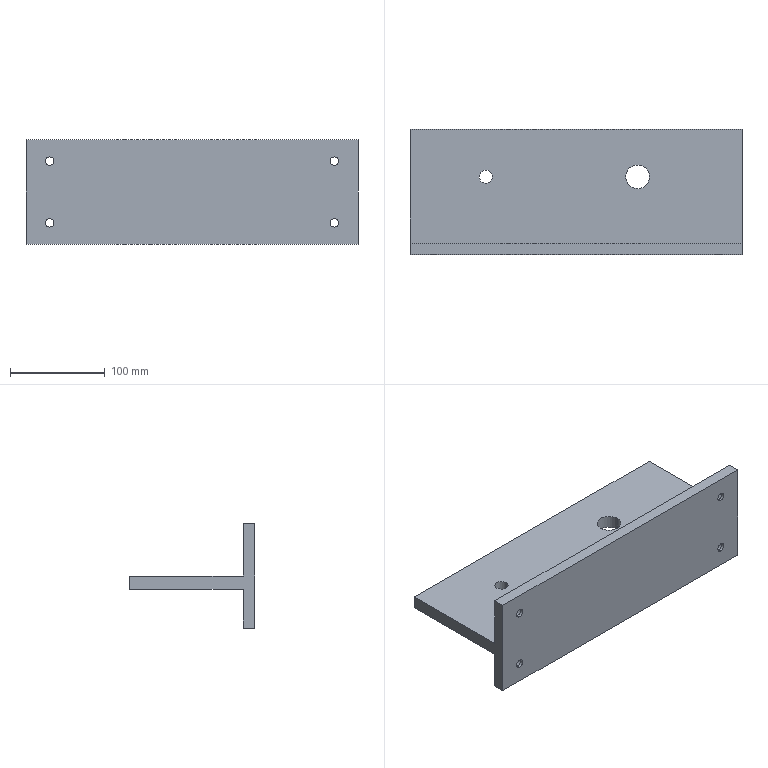Part | SolidWorks | features Cut 2, Extrusion 1, HoleWzd 1, ICE 1 | 1 solid | 42 faces | box 350 x 132 x 110 mm | volume 1033847 mm3 | cylinder 20 | plane 14 | cone 8 | commonest cylinder face diameters 9 x8 15 x8 14 x2 25 x2
STEP:
#1=CARTESIAN_POINT('',(77.5,82.,0.));
#2=VERTEX_POINT('',#1);
#3=CARTESIAN_POINT('',(52.5,82.,0.));
#4=VERTEX_POINT('',#3);
#5=CARTESIAN_POINT('',(65.,82.,0.));
#6=DIRECTION('',(0.,0.,-1.));
#7=DIRECTION('',(-1.,0.,0.));
#8=AXIS2_PLACEMENT_3D('',#5,#6,#7);
#9=CIRCLE('',#8,12.5);
#10=EDGE_CURVE('',#2,#4,#9,.T.);
#11=ORIENTED_EDGE('',*,*,#10,.F.);
#12=CARTESIAN_POINT('',(77.5,82.,-14.));
#13=VERTEX_POINT('',#12);
#14=CARTESIAN_POINT('',(77.5,82.,55.));
#15=DIRECTION('',(0.,0.,-1.));
#16=VECTOR('',#15,1000.);
#17=LINE('',#14,#16);
#18=EDGE_CURVE('',#2,#13,#17,.T.);
#19=ORIENTED_EDGE('',*,*,#18,.T.);
#20=CARTESIAN_POINT('',(52.5,82.,-14.));
#21=VERTEX_POINT('',#20);
#22=CARTESIAN_POINT('',(65.,82.,-14.));
#23=DIRECTION('',(0.,0.,1.));
#24=DIRECTION('',(1.,0.,0.));
#25=AXIS2_PLACEMENT_3D('',#22,#23,#24);
#26=CIRCLE('',#25,12.5);
#27=EDGE_CURVE('',#21,#13,#26,.T.);
#28=ORIENTED_EDGE('',*,*,#27,.F.);
#29=CARTESIAN_POINT('',(52.5,82.,55.));
#30=DIRECTION('',(0.,0.,-1.));
#31=VECTOR('',#30,1000.);
#32=LINE('',#29,#31);
#33=EDGE_CURVE('',#4,#21,#32,.T.);
#34=ORIENTED_EDGE('',*,*,#33,.F.);
#35=EDGE_LOOP('',(#11,#19,#28,#34));
#36=FACE_OUTER_BOUND('',#35,.T.);
#37=CARTESIAN_POINT('',(65.,82.,55.));
#38=DIRECTION('',(0.,0.,-1.));
#39=DIRECTION('',(-1.,0.,0.));
#40=AXIS2_PLACEMENT_3D('',#37,#38,#39);
#41=CYLINDRICAL_SURFACE('',#40,12.5);
#42=ADVANCED_FACE('',(#36),#41,.F.);
#43=CARTESIAN_POINT('',(-88.,82.,0.));
#44=VERTEX_POINT('',#43);
#45=CARTESIAN_POINT('',(-102.,82.,0.));
#46=VERTEX_POINT('',#45);
#47=CARTESIAN_POINT('',(-95.,82.,0.));
#48=DIRECTION('',(0.,0.,-1.));
#49=DIRECTION('',(-1.,0.,0.));
#50=AXIS2_PLACEMENT_3D('',#47,#48,#49);
#51=CIRCLE('',#50,7.);
#52=EDGE_CURVE('',#44,#46,#51,.T.);
#53=ORIENTED_EDGE('',*,*,#52,.F.);
#54=CARTESIAN_POINT('',(-88.,82.,-14.));
#55=VERTEX_POINT('',#54);
#56=CARTESIAN_POINT('',(-88.,82.,55.));
#57=DIRECTION('',(0.,0.,-1.));
#58=VECTOR('',#57,1000.);
#59=LINE('',#56,#58);
#60=EDGE_CURVE('',#44,#55,#59,.T.);
#61=ORIENTED_EDGE('',*,*,#60,.T.);
#62=CARTESIAN_POINT('',(-102.,82.,-14.));
#63=VERTEX_POINT('',#62);
#64=CARTESIAN_POINT('',(-95.,82.,-14.));
#65=DIRECTION('',(0.,0.,1.));
#66=DIRECTION('',(1.,0.,0.));
#67=AXIS2_PLACEMENT_3D('',#64,#65,#66);
#68=CIRCLE('',#67,7.);
#69=EDGE_CURVE('',#63,#55,#68,.T.);
#70=ORIENTED_EDGE('',*,*,#69,.F.);
#71=CARTESIAN_POINT('',(-102.,82.,55.));
#72=DIRECTION('',(0.,0.,-1.));
#73=VECTOR('',#72,1000.);
#74=LINE('',#71,#73);
#75=EDGE_CURVE('',#46,#63,#74,.T.);
#76=ORIENTED_EDGE('',*,*,#75,.F.);
#77=EDGE_LOOP('',(#53,#61,#70,#76));
#78=FACE_OUTER_BOUND('',#77,.T.);
#79=CARTESIAN_POINT('',(-95.,82.,55.));
#80=DIRECTION('',(0.,0.,-1.));
#81=DIRECTION('',(-1.,0.,0.));
#82=AXIS2_PLACEMENT_3D('',#79,#80,#81);
#83=CYLINDRICAL_SURFACE('',#82,7.);
#84=ADVANCED_FACE('',(#78),#83,.F.);
#85=CARTESIAN_POINT('',(-150.,11.975,-40.));
#86=VERTEX_POINT('',#85);
#87=CARTESIAN_POINT('',(-150.,11.975,-25.));
#88=VERTEX_POINT('',#87);
#89=CARTESIAN_POINT('',(-150.,11.975,-32.5));
#90=DIRECTION('',(0.,1.,0.));
#91=DIRECTION('',(0.,0.,1.));
#92=AXIS2_PLACEMENT_3D('',#89,#90,#91);
#93=CIRCLE('',#92,7.5);
#94=EDGE_CURVE('',#86,#88,#93,.T.);
#95=ORIENTED_EDGE('',*,*,#94,.F.);
#96=CARTESIAN_POINT('',(-150.,12.,-40.025));
#97=VERTEX_POINT('',#96);
#98=CARTESIAN_POINT('',(-150.,12.,-40.025));
#99=DIRECTION('',(0.,0.7071,-0.7071));
#100=VECTOR('',#99,1000.);
#101=LINE('',#98,#100);
#102=EDGE_CURVE('',#86,#97,#101,.T.);
#103=ORIENTED_EDGE('',*,*,#102,.T.);
#104=CARTESIAN_POINT('',(-150.,12.,-24.975));
#105=VERTEX_POINT('',#104);
#106=CARTESIAN_POINT('',(-150.,12.,-32.5));
#107=DIRECTION('',(0.,1.,0.));
#108=DIRECTION('',(0.,0.,1.));
#109=AXIS2_PLACEMENT_3D('',#106,#107,#108);
#110=CIRCLE('',#109,7.525);
#111=EDGE_CURVE('',#97,#105,#110,.T.);
#112=ORIENTED_EDGE('',*,*,#111,.T.);
#113=CARTESIAN_POINT('',(-150.,12.,-24.975));
#114=DIRECTION('',(0.,0.7071,0.7071));
#115=VECTOR('',#114,1000.);
#116=LINE('',#113,#115);
#117=EDGE_CURVE('',#88,#105,#116,.T.);
#118=ORIENTED_EDGE('',*,*,#117,.F.);
#119=EDGE_LOOP('',(#95,#103,#112,#118));
#120=FACE_OUTER_BOUND('',#119,.T.);
#121=CARTESIAN_POINT('',(-150.,12.,-32.5));
#122=DIRECTION('',(0.,1.,0.));
#123=DIRECTION('',(0.,0.,1.));
#124=AXIS2_PLACEMENT_3D('',#121,#122,#123);
#125=CONICAL_SURFACE('',#124,7.525,0.7854);
#126=ADVANCED_FACE('',(#120),#125,.F.);
#127=CARTESIAN_POINT('',(-150.,3.,-40.));
#128=VERTEX_POINT('',#127);
#129=CARTESIAN_POINT('',(-150.,3.,-25.));
#130=VERTEX_POINT('',#129);
#131=CARTESIAN_POINT('',(-150.,3.,-32.5));
#132=DIRECTION('',(0.,1.,0.));
#133=DIRECTION('',(0.,0.,1.));
#134=AXIS2_PLACEMENT_3D('',#131,#132,#133);
#135=CIRCLE('',#134,7.5);
#136=EDGE_CURVE('',#128,#130,#135,.T.);
#137=ORIENTED_EDGE('',*,*,#136,.F.);
#138=CARTESIAN_POINT('',(-150.,12.,-40.));
#139=DIRECTION('',(0.,1.,0.));
#140=VECTOR('',#139,1000.);
#141=LINE('',#138,#140);
#142=EDGE_CURVE('',#128,#86,#141,.T.);
#143=ORIENTED_EDGE('',*,*,#142,.T.);
#144=ORIENTED_EDGE('',*,*,#94,.T.);
#145=CARTESIAN_POINT('',(-150.,12.,-25.));
#146=DIRECTION('',(0.,1.,0.));
#147=VECTOR('',#146,1000.);
#148=LINE('',#145,#147);
#149=EDGE_CURVE('',#130,#88,#148,.T.);
#150=ORIENTED_EDGE('',*,*,#149,.F.);
#151=EDGE_LOOP('',(#137,#143,#144,#150));
#152=FACE_OUTER_BOUND('',#151,.T.);
#153=CARTESIAN_POINT('',(-150.,12.,-32.5));
#154=DIRECTION('',(0.,1.,0.));
#155=DIRECTION('',(0.,0.,1.));
#156=AXIS2_PLACEMENT_3D('',#153,#154,#155);
#157=CYLINDRICAL_SURFACE('',#156,7.5);
#158=ADVANCED_FACE('',(#152),#157,.F.);
#159=CARTESIAN_POINT('',(-150.,0.,-28.));
#160=VERTEX_POINT('',#159);
#161=CARTESIAN_POINT('',(-150.,0.,-37.));
#162=VERTEX_POINT('',#161);
#163=CARTESIAN_POINT('',(-150.,0.,-32.5));
#164=DIRECTION('',(0.,-1.,0.));
#165=DIRECTION('',(0.,0.,-1.));
#166=AXIS2_PLACEMENT_3D('',#163,#164,#165);
#167=CIRCLE('',#166,4.5);
#168=EDGE_CURVE('',#160,#162,#167,.T.);
#169=ORIENTED_EDGE('',*,*,#168,.T.);
#170=CARTESIAN_POINT('',(-150.,3.,-37.));
#171=VERTEX_POINT('',#170);
#172=CARTESIAN_POINT('',(-150.,12.,-37.));
#173=DIRECTION('',(0.,1.,0.));
#174=VECTOR('',#173,1000.);
#175=LINE('',#172,#174);
#176=EDGE_CURVE('',#162,#171,#175,.T.);
#177=ORIENTED_EDGE('',*,*,#176,.T.);
#178=CARTESIAN_POINT('',(-150.,3.,-28.));
#179=VERTEX_POINT('',#178);
#180=CARTESIAN_POINT('',(-150.,3.,-32.5));
#181=DIRECTION('',(0.,1.,0.));
#182=DIRECTION('',(0.,0.,1.));
#183=AXIS2_PLACEMENT_3D('',#180,#181,#182);
#184=CIRCLE('',#183,4.5);
#185=EDGE_CURVE('',#171,#179,#184,.T.);
#186=ORIENTED_EDGE('',*,*,#185,.T.);
#187=CARTESIAN_POINT('',(-150.,12.,-28.));
#188=DIRECTION('',(0.,1.,0.));
#189=VECTOR('',#188,1000.);
#190=LINE('',#187,#189);
#191=EDGE_CURVE('',#160,#179,#190,.T.);
#192=ORIENTED_EDGE('',*,*,#191,.F.);
#193=EDGE_LOOP('',(#169,#177,#186,#192));
#194=FACE_OUTER_BOUND('',#193,.T.);
#195=CARTESIAN_POINT('',(-150.,12.,-32.5));
#196=DIRECTION('',(0.,1.,0.));
#197=DIRECTION('',(0.,0.,1.));
#198=AXIS2_PLACEMENT_3D('',#195,#196,#197);
#199=CYLINDRICAL_SURFACE('',#198,4.5);
#200=ADVANCED_FACE('',(#194),#199,.F.);
#201=CARTESIAN_POINT('',(-150.,11.975,25.));
#202=VERTEX_POINT('',#201);
#203=CARTESIAN_POINT('',(-150.,11.975,40.));
#204=VERTEX_POINT('',#203);
#205=CARTESIAN_POINT('',(-150.,11.975,32.5));
#206=DIRECTION('',(0.,1.,0.));
#207=DIRECTION('',(0.,0.,1.));
#208=AXIS2_PLACEMENT_3D('',#205,#206,#207);
#209=CIRCLE('',#208,7.5);
#210=EDGE_CURVE('',#202,#204,#209,.T.);
#211=ORIENTED_EDGE('',*,*,#210,.F.);
#212=CARTESIAN_POINT('',(-150.,12.,24.975));
#213=VERTEX_POINT('',#212);
#214=CARTESIAN_POINT('',(-150.,12.,24.975));
#215=DIRECTION('',(0.,0.7071,-0.7071));
#216=VECTOR('',#215,1000.);
#217=LINE('',#214,#216);
#218=EDGE_CURVE('',#202,#213,#217,.T.);
#219=ORIENTED_EDGE('',*,*,#218,.T.);
#220=CARTESIAN_POINT('',(-150.,12.,40.025));
#221=VERTEX_POINT('',#220);
#222=CARTESIAN_POINT('',(-150.,12.,32.5));
#223=DIRECTION('',(0.,1.,0.));
#224=DIRECTION('',(0.,0.,1.));
#225=AXIS2_PLACEMENT_3D('',#222,#223,#224);
#226=CIRCLE('',#225,7.525);
#227=EDGE_CURVE('',#213,#221,#226,.T.);
#228=ORIENTED_EDGE('',*,*,#227,.T.);
#229=CARTESIAN_POINT('',(-150.,12.,40.025));
#230=DIRECTION('',(0.,0.7071,0.7071));
#231=VECTOR('',#230,1000.);
#232=LINE('',#229,#231);
#233=EDGE_CURVE('',#204,#221,#232,.T.);
#234=ORIENTED_EDGE('',*,*,#233,.F.);
#235=EDGE_LOOP('',(#211,#219,#228,#234));
#236=FACE_OUTER_BOUND('',#235,.T.);
#237=CARTESIAN_POINT('',(-150.,12.,32.5));
#238=DIRECTION('',(0.,1.,0.));
#239=DIRECTION('',(0.,0.,1.));
#240=AXIS2_PLACEMENT_3D('',#237,#238,#239);
#241=CONICAL_SURFACE('',#240,7.525,0.7854);
#242=ADVANCED_FACE('',(#236),#241,.F.);
#243=CARTESIAN_POINT('',(-150.,3.,25.));
#244=VERTEX_POINT('',#243);
#245=CARTESIAN_POINT('',(-150.,3.,40.));
#246=VERTEX_POINT('',#245);
#247=CARTESIAN_POINT('',(-150.,3.,32.5));
#248=DIRECTION('',(0.,1.,0.));
#249=DIRECTION('',(0.,0.,1.));
#250=AXIS2_PLACEMENT_3D('',#247,#248,#249);
#251=CIRCLE('',#250,7.5);
#252=EDGE_CURVE('',#244,#246,#251,.T.);
#253=ORIENTED_EDGE('',*,*,#252,.F.);
#254=CARTESIAN_POINT('',(-150.,12.,25.));
#255=DIRECTION('',(0.,1.,0.));
#256=VECTOR('',#255,1000.);
#257=LINE('',#254,#256);
#258=EDGE_CURVE('',#244,#202,#257,.T.);
#259=ORIENTED_EDGE('',*,*,#258,.T.);
#260=ORIENTED_EDGE('',*,*,#210,.T.);
#261=CARTESIAN_POINT('',(-150.,12.,40.));
#262=DIRECTION('',(0.,1.,0.));
#263=VECTOR('',#262,1000.);
#264=LINE('',#261,#263);
#265=EDGE_CURVE('',#246,#204,#264,.T.);
#266=ORIENTED_EDGE('',*,*,#265,.F.);
#267=EDGE_LOOP('',(#253,#259,#260,#266));
#268=FACE_OUTER_BOUND('',#267,.T.);
#269=CARTESIAN_POINT('',(-150.,12.,32.5));
#270=DIRECTION('',(0.,1.,0.));
#271=DIRECTION('',(0.,0.,1.));
#272=AXIS2_PLACEMENT_3D('',#269,#270,#271);
#273=CYLINDRICAL_SURFACE('',#272,7.5);
#274=ADVANCED_FACE('',(#268),#273,.F.);
#275=CARTESIAN_POINT('',(-150.,0.,37.));
#276=VERTEX_POINT('',#275);
#277=CARTESIAN_POINT('',(-150.,0.,28.));
#278=VERTEX_POINT('',#277);
#279=CARTESIAN_POINT('',(-150.,0.,32.5));
#280=DIRECTION('',(0.,-1.,0.));
#281=DIRECTION('',(0.,0.,-1.));
#282=AXIS2_PLACEMENT_3D('',#279,#280,#281);
#283=CIRCLE('',#282,4.5);
#284=EDGE_CURVE('',#276,#278,#283,.T.);
#285=ORIENTED_EDGE('',*,*,#284,.T.);
#286=CARTESIAN_POINT('',(-150.,3.,28.));
#287=VERTEX_POINT('',#286);
#288=CARTESIAN_POINT('',(-150.,12.,28.));
#289=DIRECTION('',(0.,1.,0.));
#290=VECTOR('',#289,1000.);
#291=LINE('',#288,#290);
#292=EDGE_CURVE('',#278,#287,#291,.T.);
#293=ORIENTED_EDGE('',*,*,#292,.T.);
#294=CARTESIAN_POINT('',(-150.,3.,37.));
#295=VERTEX_POINT('',#294);
#296=CARTESIAN_POINT('',(-150.,3.,32.5));
#297=DIRECTION('',(0.,1.,0.));
#298=DIRECTION('',(0.,0.,1.));
#299=AXIS2_PLACEMENT_3D('',#296,#297,#298);
#300=CIRCLE('',#299,4.5);
#301=EDGE_CURVE('',#287,#295,#300,.T.);
#302=ORIENTED_EDGE('',*,*,#301,.T.);
#303=CARTESIAN_POINT('',(-150.,12.,37.));
#304=DIRECTION('',(0.,1.,0.));
#305=VECTOR('',#304,1000.);
#306=LINE('',#303,#305);
#307=EDGE_CURVE('',#276,#295,#306,.T.);
#308=ORIENTED_EDGE('',*,*,#307,.F.);
#309=EDGE_LOOP('',(#285,#293,#302,#308));
#310=FACE_OUTER_BOUND('',#309,.T.);
#311=CARTESIAN_POINT('',(-150.,12.,32.5));
#312=DIRECTION('',(0.,1.,0.));
#313=DIRECTION('',(0.,0.,1.));
#314=AXIS2_PLACEMENT_3D('',#311,#312,#313);
#315=CYLINDRICAL_SURFACE('',#314,4.5);
#316=ADVANCED_FACE('',(#310),#315,.F.);
#317=CARTESIAN_POINT('',(150.,11.975,-40.));
#318=VERTEX_POINT('',#317);
#319=CARTESIAN_POINT('',(150.,11.975,-25.));
#320=VERTEX_POINT('',#319);
#321=CARTESIAN_POINT('',(150.,11.975,-32.5));
#322=DIRECTION('',(0.,1.,0.));
#323=DIRECTION('',(0.,0.,1.));
#324=AXIS2_PLACEMENT_3D('',#321,#322,#323);
#325=CIRCLE('',#324,7.5);
#326=EDGE_CURVE('',#318,#320,#325,.T.);
#327=ORIENTED_EDGE('',*,*,#326,.F.);
#328=CARTESIAN_POINT('',(150.,12.,-40.025));
#329=VERTEX_POINT('',#328);
#330=CARTESIAN_POINT('',(150.,12.,-40.025));
#331=DIRECTION('',(0.,0.7071,-0.7071));
#332=VECTOR('',#331,1000.);
#333=LINE('',#330,#332);
#334=EDGE_CURVE('',#318,#329,#333,.T.);
#335=ORIENTED_EDGE('',*,*,#334,.T.);
#336=CARTESIAN_POINT('',(150.,12.,-24.975));
#337=VERTEX_POINT('',#336);
#338=CARTESIAN_POINT('',(150.,12.,-32.5));
#339=DIRECTION('',(0.,1.,0.));
#340=DIRECTION('',(0.,0.,1.));
#341=AXIS2_PLACEMENT_3D('',#338,#339,#340);
#342=CIRCLE('',#341,7.525);
#343=EDGE_CURVE('',#329,#337,#342,.T.);
#344=ORIENTED_EDGE('',*,*,#343,.T.);
#345=CARTESIAN_POINT('',(150.,12.,-24.975));
#346=DIRECTION('',(0.,0.7071,0.7071));
#347=VECTOR('',#346,1000.);
#348=LINE('',#345,#347);
#349=EDGE_CURVE('',#320,#337,#348,.T.);
#350=ORIENTED_EDGE('',*,*,#349,.F.);
#351=EDGE_LOOP('',(#327,#335,#344,#350));
#352=FACE_OUTER_BOUND('',#351,.T.);
#353=CARTESIAN_POINT('',(150.,12.,-32.5));
#354=DIRECTION('',(0.,1.,0.));
#355=DIRECTION('',(0.,0.,1.));
#356=AXIS2_PLACEMENT_3D('',#353,#354,#355);
#357=CONICAL_SURFACE('',#356,7.525,0.7854);
#358=ADVANCED_FACE('',(#352),#357,.F.);
#359=CARTESIAN_POINT('',(150.,3.,-40.));
#360=VERTEX_POINT('',#359);
#361=CARTESIAN_POINT('',(150.,3.,-25.));
#362=VERTEX_POINT('',#361);
#363=CARTESIAN_POINT('',(150.,3.,-32.5));
#364=DIRECTION('',(0.,1.,0.));
#365=DIRECTION('',(0.,0.,1.));
#366=AXIS2_PLACEMENT_3D('',#363,#364,#365);
#367=CIRCLE('',#366,7.5);
#368=EDGE_CURVE('',#360,#362,#367,.T.);
#369=ORIENTED_EDGE('',*,*,#368,.F.);
#370=CARTESIAN_POINT('',(150.,12.,-40.));
#371=DIRECTION('',(0.,1.,0.));
#372=VECTOR('',#371,1000.);
#373=LINE('',#370,#372);
#374=EDGE_CURVE('',#360,#318,#373,.T.);
#375=ORIENTED_EDGE('',*,*,#374,.T.);
#376=ORIENTED_EDGE('',*,*,#326,.T.);
#377=CARTESIAN_POINT('',(150.,12.,-25.));
#378=DIRECTION('',(0.,1.,0.));
#379=VECTOR('',#378,1000.);
#380=LINE('',#377,#379);
#381=EDGE_CURVE('',#362,#320,#380,.T.);
#382=ORIENTED_EDGE('',*,*,#381,.F.);
#383=EDGE_LOOP('',(#369,#375,#376,#382));
#384=FACE_OUTER_BOUND('',#383,.T.);
#385=CARTESIAN_POINT('',(150.,12.,-32.5));
#386=DIRECTION('',(0.,1.,0.));
#387=DIRECTION('',(0.,0.,1.));
#388=AXIS2_PLACEMENT_3D('',#385,#386,#387);
#389=CYLINDRICAL_SURFACE('',#388,7.5);
#390=ADVANCED_FACE('',(#384),#389,.F.);
#391=CARTESIAN_POINT('',(150.,0.,-28.));
#392=VERTEX_POINT('',#391);
#393=CARTESIAN_POINT('',(150.,0.,-37.));
#394=VERTEX_POINT('',#393);
#395=CARTESIAN_POINT('',(150.,0.,-32.5));
#396=DIRECTION('',(0.,-1.,0.));
#397=DIRECTION('',(0.,0.,-1.));
#398=AXIS2_PLACEMENT_3D('',#395,#396,#397);
#399=CIRCLE('',#398,4.5);
#400=EDGE_CURVE('',#392,#394,#399,.T.);
#401=ORIENTED_EDGE('',*,*,#400,.T.);
#402=CARTESIAN_POINT('',(150.,3.,-37.));
#403=VERTEX_POINT('',#402);
#404=CARTESIAN_POINT('',(150.,12.,-37.));
#405=DIRECTION('',(0.,1.,0.));
#406=VECTOR('',#405,1000.);
#407=LINE('',#404,#406);
#408=EDGE_CURVE('',#394,#403,#407,.T.);
#409=ORIENTED_EDGE('',*,*,#408,.T.);
#410=CARTESIAN_POINT('',(150.,3.,-28.));
#411=VERTEX_POINT('',#410);
#412=CARTESIAN_POINT('',(150.,3.,-32.5));
#413=DIRECTION('',(0.,1.,0.));
#414=DIRECTION('',(0.,0.,1.));
#415=AXIS2_PLACEMENT_3D('',#412,#413,#414);
#416=CIRCLE('',#415,4.5);
#417=EDGE_CURVE('',#403,#411,#416,.T.);
#418=ORIENTED_EDGE('',*,*,#417,.T.);
#419=CARTESIAN_POINT('',(150.,12.,-28.));
#420=DIRECTION('',(0.,1.,0.));
#421=VECTOR('',#420,1000.);
#422=LINE('',#419,#421);
#423=EDGE_CURVE('',#392,#411,#422,.T.);
#424=ORIENTED_EDGE('',*,*,#423,.F.);
#425=EDGE_LOOP('',(#401,#409,#418,#424));
#426=FACE_OUTER_BOUND('',#425,.T.);
#427=CARTESIAN_POINT('',(150.,12.,-32.5));
#428=DIRECTION('',(0.,1.,0.));
#429=DIRECTION('',(0.,0.,1.));
#430=AXIS2_PLACEMENT_3D('',#427,#428,#429);
#431=CYLINDRICAL_SURFACE('',#430,4.5);
#432=ADVANCED_FACE('',(#426),#431,.F.);
#433=CARTESIAN_POINT('',(150.,11.975,25.));
#434=VERTEX_POINT('',#433);
#435=CARTESIAN_POINT('',(150.,11.975,40.));
#436=VERTEX_POINT('',#435);
#437=CARTESIAN_POINT('',(150.,11.975,32.5));
#438=DIRECTION('',(0.,1.,0.));
#439=DIRECTION('',(0.,0.,1.));
#440=AXIS2_PLACEMENT_3D('',#437,#438,#439);
#441=CIRCLE('',#440,7.5);
#442=EDGE_CURVE('',#434,#436,#441,.T.);
#443=ORIENTED_EDGE('',*,*,#442,.F.);
#444=CARTESIAN_POINT('',(150.,12.,24.975));
#445=VERTEX_POINT('',#444);
#446=CARTESIAN_POINT('',(150.,12.,24.975));
#447=DIRECTION('',(0.,0.7071,-0.7071));
#448=VECTOR('',#447,1000.);
#449=LINE('',#446,#448);
#450=EDGE_CURVE('',#434,#445,#449,.T.);
#451=ORIENTED_EDGE('',*,*,#450,.T.);
#452=CARTESIAN_POINT('',(150.,12.,40.025));
#453=VERTEX_POINT('',#452);
#454=CARTESIAN_POINT('',(150.,12.,32.5));
#455=DIRECTION('',(0.,1.,0.));
#456=DIRECTION('',(0.,0.,1.));
#457=AXIS2_PLACEMENT_3D('',#454,#455,#456);
#458=CIRCLE('',#457,7.525);
#459=EDGE_CURVE('',#445,#453,#458,.T.);
#460=ORIENTED_EDGE('',*,*,#459,.T.);
#461=CARTESIAN_POINT('',(150.,12.,40.025));
#462=DIRECTION('',(0.,0.7071,0.7071));
#463=VECTOR('',#462,1000.);
#464=LINE('',#461,#463);
#465=EDGE_CURVE('',#436,#453,#464,.T.);
#466=ORIENTED_EDGE('',*,*,#465,.F.);
#467=EDGE_LOOP('',(#443,#451,#460,#466));
#468=FACE_OUTER_BOUND('',#467,.T.);
#469=CARTESIAN_POINT('',(150.,12.,32.5));
#470=DIRECTION('',(0.,1.,0.));
#471=DIRECTION('',(0.,0.,1.));
#472=AXIS2_PLACEMENT_3D('',#469,#470,#471);
#473=CONICAL_SURFACE('',#472,7.525,0.7854);
#474=ADVANCED_FACE('',(#468),#473,.F.);
#475=CARTESIAN_POINT('',(150.,3.,25.));
#476=VERTEX_POINT('',#475);
#477=CARTESIAN_POINT('',(150.,3.,40.));
#478=VERTEX_POINT('',#477);
#479=CARTESIAN_POINT('',(150.,3.,32.5));
#480=DIRECTION('',(0.,1.,0.));
#481=DIRECTION('',(0.,0.,1.));
#482=AXIS2_PLACEMENT_3D('',#479,#480,#481);
#483=CIRCLE('',#482,7.5);
#484=EDGE_CURVE('',#476,#478,#483,.T.);
#485=ORIENTED_EDGE('',*,*,#484,.F.);
#486=CARTESIAN_POINT('',(150.,12.,25.));
#487=DIRECTION('',(0.,1.,0.));
#488=VECTOR('',#487,1000.);
#489=LINE('',#486,#488);
#490=EDGE_CURVE('',#476,#434,#489,.T.);
#491=ORIENTED_EDGE('',*,*,#490,.T.);
#492=ORIENTED_EDGE('',*,*,#442,.T.);
#493=CARTESIAN_POINT('',(150.,12.,40.));
#494=DIRECTION('',(0.,1.,0.));
#495=VECTOR('',#494,1000.);
#496=LINE('',#493,#495);
#497=EDGE_CURVE('',#478,#436,#496,.T.);
#498=ORIENTED_EDGE('',*,*,#497,.F.);
#499=EDGE_LOOP('',(#485,#491,#492,#498));
#500=FACE_OUTER_BOUND('',#499,.T.);
#501=CARTESIAN_POINT('',(150.,12.,32.5));
#502=DIRECTION('',(0.,1.,0.));
#503=DIRECTION('',(0.,0.,1.));
#504=AXIS2_PLACEMENT_3D('',#501,#502,#503);
#505=CYLINDRICAL_SURFACE('',#504,7.5);
#506=ADVANCED_FACE('',(#500),#505,.F.);
#507=CARTESIAN_POINT('',(150.,0.,37.));
#508=VERTEX_POINT('',#507);
#509=CARTESIAN_POINT('',(150.,0.,28.));
#510=VERTEX_POINT('',#509);
#511=CARTESIAN_POINT('',(150.,0.,32.5));
#512=DIRECTION('',(0.,-1.,0.));
#513=DIRECTION('',(0.,0.,-1.));
#514=AXIS2_PLACEMENT_3D('',#511,#512,#513);
#515=CIRCLE('',#514,4.5);
#516=EDGE_CURVE('',#508,#510,#515,.T.);
#517=ORIENTED_EDGE('',*,*,#516,.T.);
#518=CARTESIAN_POINT('',(150.,3.,28.));
#519=VERTEX_POINT('',#518);
#520=CARTESIAN_POINT('',(150.,12.,28.));
#521=DIRECTION('',(0.,1.,0.));
#522=VECTOR('',#521,1000.);
#523=LINE('',#520,#522);
#524=EDGE_CURVE('',#510,#519,#523,.T.);
#525=ORIENTED_EDGE('',*,*,#524,.T.);
#526=CARTESIAN_POINT('',(150.,3.,37.));
#527=VERTEX_POINT('',#526);
#528=CARTESIAN_POINT('',(150.,3.,32.5));
#529=DIRECTION('',(0.,1.,0.));
#530=DIRECTION('',(0.,0.,1.));
#531=AXIS2_PLACEMENT_3D('',#528,#529,#530);
#532=CIRCLE('',#531,4.5);
#533=EDGE_CURVE('',#519,#527,#532,.T.);
#534=ORIENTED_EDGE('',*,*,#533,.T.);
#535=CARTESIAN_POINT('',(150.,12.,37.));
#536=DIRECTION('',(0.,1.,0.));
#537=VECTOR('',#536,1000.);
#538=LINE('',#535,#537);
#539=EDGE_CURVE('',#508,#527,#538,.T.);
#540=ORIENTED_EDGE('',*,*,#539,.F.);
#541=EDGE_LOOP('',(#517,#525,#534,#540));
#542=FACE_OUTER_BOUND('',#541,.T.);
#543=CARTESIAN_POINT('',(150.,12.,32.5));
#544=DIRECTION('',(0.,1.,0.));
#545=DIRECTION('',(0.,0.,1.));
#546=AXIS2_PLACEMENT_3D('',#543,#544,#545);
#547=CYLINDRICAL_SURFACE('',#546,4.5);
#548=ADVANCED_FACE('',(#542),#547,.F.);
#549=CARTESIAN_POINT('',(-150.,12.,-32.5));
#550=DIRECTION('',(0.,1.,0.));
#551=DIRECTION('',(0.,0.,1.));
#552=AXIS2_PLACEMENT_3D('',#549,#550,#551);
#553=CIRCLE('',#552,7.525);
#554=EDGE_CURVE('',#105,#97,#553,.T.);
#555=ORIENTED_EDGE('',*,*,#554,.F.);
#556=ORIENTED_EDGE('',*,*,#111,.F.);
#557=EDGE_LOOP('',(#555,#556));
#558=FACE_BOUND('',#557,.T.);
#559=CARTESIAN_POINT('',(150.,12.,-32.5));
#560=DIRECTION('',(0.,1.,0.));
#561=DIRECTION('',(0.,0.,1.));
#562=AXIS2_PLACEMENT_3D('',#559,#560,#561);
#563=CIRCLE('',#562,7.525);
#564=EDGE_CURVE('',#337,#329,#563,.T.);
#565=ORIENTED_EDGE('',*,*,#564,.F.);
#566=ORIENTED_EDGE('',*,*,#343,.F.);
#567=EDGE_LOOP('',(#565,#566));
#568=FACE_BOUND('',#567,.T.);
#569=CARTESIAN_POINT('',(175.,12.,-14.));
#570=VERTEX_POINT('',#569);
#571=CARTESIAN_POINT('',(-175.,12.,-14.));
#572=VERTEX_POINT('',#571);
#573=CARTESIAN_POINT('',(-175.,12.,-14.));
#574=DIRECTION('',(-1.,0.,0.));
#575=VECTOR('',#574,1000.);
#576=LINE('',#573,#575);
#577=EDGE_CURVE('',#570,#572,#576,.T.);
#578=ORIENTED_EDGE('',*,*,#577,.F.);
#579=CARTESIAN_POINT('',(175.,12.,-55.));
#580=VERTEX_POINT('',#579);
#581=CARTESIAN_POINT('',(175.,12.,55.));
#582=DIRECTION('',(0.,0.,-1.));
#583=VECTOR('',#582,1000.);
#584=LINE('',#581,#583);
#585=EDGE_CURVE('',#570,#580,#584,.T.);
#586=ORIENTED_EDGE('',*,*,#585,.T.);
#587=CARTESIAN_POINT('',(-175.,12.,-55.));
#588=VERTEX_POINT('',#587);
#589=CARTESIAN_POINT('',(-175.,12.,-55.));
#590=DIRECTION('',(-1.,0.,0.));
#591=VECTOR('',#590,1000.);
#592=LINE('',#589,#591);
#593=EDGE_CURVE('',#580,#588,#592,.T.);
#594=ORIENTED_EDGE('',*,*,#593,.T.);
#595=CARTESIAN_POINT('',(-175.,12.,55.));
#596=DIRECTION('',(0.,0.,1.));
#597=VECTOR('',#596,1000.);
#598=LINE('',#595,#597);
#599=EDGE_CURVE('',#588,#572,#598,.T.);
#600=ORIENTED_EDGE('',*,*,#599,.T.);
#601=EDGE_LOOP('',(#578,#586,#594,#600));
#602=FACE_OUTER_BOUND('',#601,.T.);
#603=CARTESIAN_POINT('',(0.,12.,0.));
#604=DIRECTION('',(0.,-1.,0.));
#605=DIRECTION('',(0.,0.,-1.));
#606=AXIS2_PLACEMENT_3D('',#603,#604,#605);
#607=PLANE('',#606);
#608=ADVANCED_FACE('',(#558,#568,#602),#607,.F.);
#609=CARTESIAN_POINT('',(-150.,12.,32.5));
#610=DIRECTION('',(0.,1.,0.));
#611=DIRECTION('',(0.,0.,1.));
#612=AXIS2_PLACEMENT_3D('',#609,#610,#611);
#613=CIRCLE('',#612,7.525);
#614=EDGE_CURVE('',#221,#213,#613,.T.);
#615=ORIENTED_EDGE('',*,*,#614,.F.);
#616=ORIENTED_EDGE('',*,*,#227,.F.);
#617=EDGE_LOOP('',(#615,#616));
#618=FACE_BOUND('',#617,.T.);
#619=CARTESIAN_POINT('',(150.,12.,32.5));
#620=DIRECTION('',(0.,1.,0.));
#621=DIRECTION('',(0.,0.,1.));
#622=AXIS2_PLACEMENT_3D('',#619,#620,#621);
#623=CIRCLE('',#622,7.525);
#624=EDGE_CURVE('',#453,#445,#623,.T.);
#625=ORIENTED_EDGE('',*,*,#624,.F.);
#626=ORIENTED_EDGE('',*,*,#459,.F.);
#627=EDGE_LOOP('',(#625,#626));
#628=FACE_BOUND('',#627,.T.);
#629=CARTESIAN_POINT('',(-175.,12.,0.));
#630=VERTEX_POINT('',#629);
#631=CARTESIAN_POINT('',(175.,12.,0.));
#632=VERTEX_POINT('',#631);
#633=CARTESIAN_POINT('',(-175.,12.,0.));
#634=DIRECTION('',(1.,0.,0.));
#635=VECTOR('',#634,1000.);
#636=LINE('',#633,#635);
#637=EDGE_CURVE('',#630,#632,#636,.T.);
#638=ORIENTED_EDGE('',*,*,#637,.F.);
#639=CARTESIAN_POINT('',(-175.,12.,55.));
#640=VERTEX_POINT('',#639);
#641=CARTESIAN_POINT('',(-175.,12.,55.));
#642=DIRECTION('',(0.,0.,1.));
#643=VECTOR('',#642,1000.);
#644=LINE('',#641,#643);
#645=EDGE_CURVE('',#630,#640,#644,.T.);
#646=ORIENTED_EDGE('',*,*,#645,.T.);
#647=CARTESIAN_POINT('',(175.,12.,55.));
#648=VERTEX_POINT('',#647);
#649=CARTESIAN_POINT('',(-175.,12.,55.));
#650=DIRECTION('',(1.,0.,0.));
#651=VECTOR('',#650,1000.);
#652=LINE('',#649,#651);
#653=EDGE_CURVE('',#640,#648,#652,.T.);
#654=ORIENTED_EDGE('',*,*,#653,.T.);
#655=CARTESIAN_POINT('',(175.,12.,55.));
#656=DIRECTION('',(0.,0.,-1.));
#657=VECTOR('',#656,1000.);
#658=LINE('',#655,#657);
#659=EDGE_CURVE('',#648,#632,#658,.T.);
#660=ORIENTED_EDGE('',*,*,#659,.T.);
#661=EDGE_LOOP('',(#638,#646,#654,#660));
#662=FACE_OUTER_BOUND('',#661,.T.);
#663=CARTESIAN_POINT('',(0.,12.,0.));
#664=DIRECTION('',(0.,-1.,0.));
#665=DIRECTION('',(0.,0.,-1.));
#666=AXIS2_PLACEMENT_3D('',#663,#664,#665);
#667=PLANE('',#666);
#668=ADVANCED_FACE('',(#618,#628,#662),#667,.F.);
#669=CARTESIAN_POINT('',(175.,0.,55.));
#670=VERTEX_POINT('',#669);
#671=CARTESIAN_POINT('',(175.,0.,-55.));
#672=VERTEX_POINT('',#671);
#673=CARTESIAN_POINT('',(175.,0.,55.));
#674=DIRECTION('',(0.,0.,-1.));
#675=VECTOR('',#674,1000.);
#676=LINE('',#673,#675);
#677=EDGE_CURVE('',#670,#672,#676,.T.);
#678=ORIENTED_EDGE('',*,*,#677,.T.);
#679=CARTESIAN_POINT('',(175.,12.,-55.));
#680=DIRECTION('',(0.,-1.,0.));
#681=VECTOR('',#680,1000.);
#682=LINE('',#679,#681);
#683=EDGE_CURVE('',#580,#672,#682,.T.);
#684=ORIENTED_EDGE('',*,*,#683,.F.);
#685=ORIENTED_EDGE('',*,*,#585,.F.);
#686=CARTESIAN_POINT('',(175.,132.,-14.));
#687=VERTEX_POINT('',#686);
#688=CARTESIAN_POINT('',(175.,132.,-14.));
#689=DIRECTION('',(0.,-1.,0.));
#690=VECTOR('',#689,1000.);
#691=LINE('',#688,#690);
#692=EDGE_CURVE('',#687,#570,#691,.T.);
#693=ORIENTED_EDGE('',*,*,#692,.F.);
#694=CARTESIAN_POINT('',(175.,132.,0.));
#695=VERTEX_POINT('',#694);
#696=CARTESIAN_POINT('',(175.,132.,-14.));
#697=DIRECTION('',(0.,0.,-1.));
#698=VECTOR('',#697,1000.);
#699=LINE('',#696,#698);
#700=EDGE_CURVE('',#695,#687,#699,.T.);
#701=ORIENTED_EDGE('',*,*,#700,.F.);
#702=CARTESIAN_POINT('',(175.,132.,0.));
#703=DIRECTION('',(0.,-1.,0.));
#704=VECTOR('',#703,1000.);
#705=LINE('',#702,#704);
#706=EDGE_CURVE('',#695,#632,#705,.T.);
#707=ORIENTED_EDGE('',*,*,#706,.T.);
#708=ORIENTED_EDGE('',*,*,#659,.F.);
#709=CARTESIAN_POINT('',(175.,12.,55.));
#710=DIRECTION('',(0.,-1.,0.));
#711=VECTOR('',#710,1000.);
#712=LINE('',#709,#711);
#713=EDGE_CURVE('',#648,#670,#712,.T.);
#714=ORIENTED_EDGE('',*,*,#713,.T.);
#715=EDGE_LOOP('',(#678,#684,#685,#693,#701,#707,#708,#714));
#716=FACE_OUTER_BOUND('',#715,.T.);
#717=CARTESIAN_POINT('',(175.,12.,55.));
#718=DIRECTION('',(-1.,0.,0.));
#719=DIRECTION('',(0.,0.,1.));
#720=AXIS2_PLACEMENT_3D('',#717,#718,#719);
#721=PLANE('',#720);
#722=ADVANCED_FACE('',(#716),#721,.F.);
#723=CARTESIAN_POINT('',(-175.,0.,-55.));
#724=VERTEX_POINT('',#723);
#725=CARTESIAN_POINT('',(-175.,0.,-55.));
#726=DIRECTION('',(-1.,0.,0.));
#727=VECTOR('',#726,1000.);
#728=LINE('',#725,#727);
#729=EDGE_CURVE('',#672,#724,#728,.T.);
#730=ORIENTED_EDGE('',*,*,#729,.T.);
#731=CARTESIAN_POINT('',(-175.,12.,-55.));
#732=DIRECTION('',(0.,-1.,0.));
#733=VECTOR('',#732,1000.);
#734=LINE('',#731,#733);
#735=EDGE_CURVE('',#588,#724,#734,.T.);
#736=ORIENTED_EDGE('',*,*,#735,.F.);
#737=ORIENTED_EDGE('',*,*,#593,.F.);
#738=ORIENTED_EDGE('',*,*,#683,.T.);
#739=EDGE_LOOP('',(#730,#736,#737,#738));
#740=FACE_OUTER_BOUND('',#739,.T.);
#741=CARTESIAN_POINT('',(-175.,12.,-55.));
#742=DIRECTION('',(0.,0.,1.));
#743=DIRECTION('',(1.,0.,0.));
#744=AXIS2_PLACEMENT_3D('',#741,#742,#743);
#745=PLANE('',#744);
#746=ADVANCED_FACE('',(#740),#745,.F.);
#747=CARTESIAN_POINT('',(-175.,0.,55.));
#748=VERTEX_POINT('',#747);
#749=CARTESIAN_POINT('',(-175.,0.,55.));
#750=DIRECTION('',(0.,0.,1.));
#751=VECTOR('',#750,1000.);
#752=LINE('',#749,#751);
#753=EDGE_CURVE('',#724,#748,#752,.T.);
#754=ORIENTED_EDGE('',*,*,#753,.T.);
#755=CARTESIAN_POINT('',(-175.,12.,55.));
#756=DIRECTION('',(0.,-1.,0.));
#757=VECTOR('',#756,1000.);
#758=LINE('',#755,#757);
#759=EDGE_CURVE('',#640,#748,#758,.T.);
#760=ORIENTED_EDGE('',*,*,#759,.F.);
#761=ORIENTED_EDGE('',*,*,#645,.F.);
#762=CARTESIAN_POINT('',(-175.,132.,0.));
#763=VERTEX_POINT('',#762);
#764=CARTESIAN_POINT('',(-175.,132.,0.));
#765=DIRECTION('',(0.,-1.,0.));
#766=VECTOR('',#765,1000.);
#767=LINE('',#764,#766);
#768=EDGE_CURVE('',#763,#630,#767,.T.);
#769=ORIENTED_EDGE('',*,*,#768,.F.);
#770=CARTESIAN_POINT('',(-175.,132.,-14.));
#771=VERTEX_POINT('',#770);
#772=CARTESIAN_POINT('',(-175.,132.,-14.));
#773=DIRECTION('',(0.,0.,1.));
#774=VECTOR('',#773,1000.);
#775=LINE('',#772,#774);
#776=EDGE_CURVE('',#771,#763,#775,.T.);
#777=ORIENTED_EDGE('',*,*,#776,.F.);
#778=CARTESIAN_POINT('',(-175.,132.,-14.));
#779=DIRECTION('',(0.,-1.,0.));
#780=VECTOR('',#779,1000.);
#781=LINE('',#778,#780);
#782=EDGE_CURVE('',#771,#572,#781,.T.);
#783=ORIENTED_EDGE('',*,*,#782,.T.);
#784=ORIENTED_EDGE('',*,*,#599,.F.);
#785=ORIENTED_EDGE('',*,*,#735,.T.);
#786=EDGE_LOOP('',(#754,#760,#761,#769,#777,#783,#784,#785));
#787=FACE_OUTER_BOUND('',#786,.T.);
#788=CARTESIAN_POINT('',(-175.,12.,55.));
#789=DIRECTION('',(1.,0.,0.));
#790=DIRECTION('',(0.,0.,-1.));
#791=AXIS2_PLACEMENT_3D('',#788,#789,#790);
#792=PLANE('',#791);
#793=ADVANCED_FACE('',(#787),#792,.F.);
#794=CARTESIAN_POINT('',(-175.,0.,55.));
#795=DIRECTION('',(1.,0.,0.));
#796=VECTOR('',#795,1000.);
#797=LINE('',#794,#796);
#798=EDGE_CURVE('',#748,#670,#797,.T.);
#799=ORIENTED_EDGE('',*,*,#798,.T.);
#800=ORIENTED_EDGE('',*,*,#713,.F.);
#801=ORIENTED_EDGE('',*,*,#653,.F.);
#802=ORIENTED_EDGE('',*,*,#759,.T.);
#803=EDGE_LOOP('',(#799,#800,#801,#802));
#804=FACE_OUTER_BOUND('',#803,.T.);
#805=CARTESIAN_POINT('',(-175.,12.,55.));
#806=DIRECTION('',(0.,0.,-1.));
#807=DIRECTION('',(-1.,0.,0.));
#808=AXIS2_PLACEMENT_3D('',#805,#806,#807);
#809=PLANE('',#808);
#810=ADVANCED_FACE('',(#804),#809,.F.);
#811=ORIENTED_EDGE('',*,*,#168,.F.);
#812=CARTESIAN_POINT('',(-150.,0.,-32.5));
#813=DIRECTION('',(0.,-1.,0.));
#814=DIRECTION('',(0.,0.,-1.));
#815=AXIS2_PLACEMENT_3D('',#812,#813,#814);
#816=CIRCLE('',#815,4.5);
#817=EDGE_CURVE('',#162,#160,#816,.T.);
#818=ORIENTED_EDGE('',*,*,#817,.F.);
#819=EDGE_LOOP('',(#811,#818));
#820=FACE_BOUND('',#819,.T.);
#821=ORIENTED_EDGE('',*,*,#284,.F.);
#822=CARTESIAN_POINT('',(-150.,0.,32.5));
#823=DIRECTION('',(0.,-1.,0.));
#824=DIRECTION('',(0.,0.,-1.));
#825=AXIS2_PLACEMENT_3D('',#822,#823,#824);
#826=CIRCLE('',#825,4.5);
#827=EDGE_CURVE('',#278,#276,#826,.T.);
#828=ORIENTED_EDGE('',*,*,#827,.F.);
#829=EDGE_LOOP('',(#821,#828));
#830=FACE_BOUND('',#829,.T.);
#831=ORIENTED_EDGE('',*,*,#400,.F.);
#832=CARTESIAN_POINT('',(150.,0.,-32.5));
#833=DIRECTION('',(0.,-1.,0.));
#834=DIRECTION('',(0.,0.,-1.));
#835=AXIS2_PLACEMENT_3D('',#832,#833,#834);
#836=CIRCLE('',#835,4.5);
#837=EDGE_CURVE('',#394,#392,#836,.T.);
#838=ORIENTED_EDGE('',*,*,#837,.F.);
#839=EDGE_LOOP('',(#831,#838));
#840=FACE_BOUND('',#839,.T.);
#841=ORIENTED_EDGE('',*,*,#516,.F.);
#842=CARTESIAN_POINT('',(150.,0.,32.5));
#843=DIRECTION('',(0.,-1.,0.));
#844=DIRECTION('',(0.,0.,-1.));
#845=AXIS2_PLACEMENT_3D('',#842,#843,#844);
#846=CIRCLE('',#845,4.5);
#847=EDGE_CURVE('',#510,#508,#846,.T.);
#848=ORIENTED_EDGE('',*,*,#847,.F.);
#849=EDGE_LOOP('',(#841,#848));
#850=FACE_BOUND('',#849,.T.);
#851=ORIENTED_EDGE('',*,*,#677,.F.);
#852=ORIENTED_EDGE('',*,*,#798,.F.);
#853=ORIENTED_EDGE('',*,*,#753,.F.);
#854=ORIENTED_EDGE('',*,*,#729,.F.);
#855=EDGE_LOOP('',(#851,#852,#853,#854));
#856=FACE_OUTER_BOUND('',#855,.T.);
#857=CARTESIAN_POINT('',(0.,0.,0.));
#858=DIRECTION('',(0.,-1.,0.));
#859=DIRECTION('',(0.,0.,-1.));
#860=AXIS2_PLACEMENT_3D('',#857,#858,#859);
#861=PLANE('',#860);
#862=ADVANCED_FACE('',(#820,#830,#840,#850,#856),#861,.T.);
#863=CARTESIAN_POINT('',(65.,82.,0.));
#864=DIRECTION('',(0.,0.,-1.));
#865=DIRECTION('',(-1.,0.,0.));
#866=AXIS2_PLACEMENT_3D('',#863,#864,#865);
#867=CIRCLE('',#866,12.5);
#868=EDGE_CURVE('',#4,#2,#867,.T.);
#869=ORIENTED_EDGE('',*,*,#868,.T.);
#870=ORIENTED_EDGE('',*,*,#10,.T.);
#871=EDGE_LOOP('',(#869,#870));
#872=FACE_BOUND('',#871,.T.);
#873=CARTESIAN_POINT('',(-95.,82.,0.));
#874=DIRECTION('',(0.,0.,-1.));
#875=DIRECTION('',(-1.,0.,0.));
#876=AXIS2_PLACEMENT_3D('',#873,#874,#875);
#877=CIRCLE('',#876,7.);
#878=EDGE_CURVE('',#46,#44,#877,.T.);
#879=ORIENTED_EDGE('',*,*,#878,.T.);
#880=ORIENTED_EDGE('',*,*,#52,.T.);
#881=EDGE_LOOP('',(#879,#880));
#882=FACE_BOUND('',#881,.T.);
#883=ORIENTED_EDGE('',*,*,#637,.T.);
#884=ORIENTED_EDGE('',*,*,#706,.F.);
#885=CARTESIAN_POINT('',(-175.,132.,0.));
#886=DIRECTION('',(1.,0.,0.));
#887=VECTOR('',#886,1000.);
#888=LINE('',#885,#887);
#889=EDGE_CURVE('',#763,#695,#888,.T.);
#890=ORIENTED_EDGE('',*,*,#889,.F.);
#891=ORIENTED_EDGE('',*,*,#768,.T.);
#892=EDGE_LOOP('',(#883,#884,#890,#891));
#893=FACE_OUTER_BOUND('',#892,.T.);
#894=CARTESIAN_POINT('',(-175.,132.,0.));
#895=DIRECTION('',(0.,0.,-1.));
#896=DIRECTION('',(-1.,0.,0.));
#897=AXIS2_PLACEMENT_3D('',#894,#895,#896);
#898=PLANE('',#897);
#899=ADVANCED_FACE('',(#872,#882,#893),#898,.F.);
#900=ORIENTED_EDGE('',*,*,#27,.T.);
#901=CARTESIAN_POINT('',(65.,82.,-14.));
#902=DIRECTION('',(0.,0.,1.));
#903=DIRECTION('',(1.,0.,0.));
#904=AXIS2_PLACEMENT_3D('',#901,#902,#903);
#905=CIRCLE('',#904,12.5);
#906=EDGE_CURVE('',#13,#21,#905,.T.);
#907=ORIENTED_EDGE('',*,*,#906,.T.);
#908=EDGE_LOOP('',(#900,#907));
#909=FACE_BOUND('',#908,.T.);
#910=ORIENTED_EDGE('',*,*,#69,.T.);
#911=CARTESIAN_POINT('',(-95.,82.,-14.));
#912=DIRECTION('',(0.,0.,1.));
#913=DIRECTION('',(1.,0.,0.));
#914=AXIS2_PLACEMENT_3D('',#911,#912,#913);
#915=CIRCLE('',#914,7.);
#916=EDGE_CURVE('',#55,#63,#915,.T.);
#917=ORIENTED_EDGE('',*,*,#916,.T.);
#918=EDGE_LOOP('',(#910,#917));
#919=FACE_BOUND('',#918,.T.);
#920=ORIENTED_EDGE('',*,*,#577,.T.);
#921=ORIENTED_EDGE('',*,*,#782,.F.);
#922=CARTESIAN_POINT('',(-175.,132.,-14.));
#923=DIRECTION('',(-1.,0.,0.));
#924=VECTOR('',#923,1000.);
#925=LINE('',#922,#924);
#926=EDGE_CURVE('',#687,#771,#925,.T.);
#927=ORIENTED_EDGE('',*,*,#926,.F.);
#928=ORIENTED_EDGE('',*,*,#692,.T.);
#929=EDGE_LOOP('',(#920,#921,#927,#928));
#930=FACE_OUTER_BOUND('',#929,.T.);
#931=CARTESIAN_POINT('',(-175.,132.,-14.));
#932=DIRECTION('',(0.,0.,1.));
#933=DIRECTION('',(1.,0.,0.));
#934=AXIS2_PLACEMENT_3D('',#931,#932,#933);
#935=PLANE('',#934);
#936=ADVANCED_FACE('',(#909,#919,#930),#935,.F.);
#937=ORIENTED_EDGE('',*,*,#776,.T.);
#938=ORIENTED_EDGE('',*,*,#889,.T.);
#939=ORIENTED_EDGE('',*,*,#700,.T.);
#940=ORIENTED_EDGE('',*,*,#926,.T.);
#941=EDGE_LOOP('',(#937,#938,#939,#940));
#942=FACE_OUTER_BOUND('',#941,.T.);
#943=CARTESIAN_POINT('',(0.,132.,0.));
#944=DIRECTION('',(0.,1.,0.));
#945=DIRECTION('',(0.,0.,1.));
#946=AXIS2_PLACEMENT_3D('',#943,#944,#945);
#947=PLANE('',#946);
#948=ADVANCED_FACE('',(#942),#947,.T.);
#949=ORIENTED_EDGE('',*,*,#524,.F.);
#950=ORIENTED_EDGE('',*,*,#847,.T.);
#951=ORIENTED_EDGE('',*,*,#539,.T.);
#952=CARTESIAN_POINT('',(150.,3.,32.5));
#953=DIRECTION('',(0.,1.,0.));
#954=DIRECTION('',(0.,0.,1.));
#955=AXIS2_PLACEMENT_3D('',#952,#953,#954);
#956=CIRCLE('',#955,4.5);
#957=EDGE_CURVE('',#527,#519,#956,.T.);
#958=ORIENTED_EDGE('',*,*,#957,.T.);
#959=EDGE_LOOP('',(#949,#950,#951,#958));
#960=FACE_OUTER_BOUND('',#959,.T.);
#961=CARTESIAN_POINT('',(150.,12.,32.5));
#962=DIRECTION('',(0.,1.,0.));
#963=DIRECTION('',(0.,0.,1.));
#964=AXIS2_PLACEMENT_3D('',#961,#962,#963);
#965=CYLINDRICAL_SURFACE('',#964,4.5);
#966=ADVANCED_FACE('',(#960),#965,.F.);
#967=ORIENTED_EDGE('',*,*,#957,.F.);
#968=ORIENTED_EDGE('',*,*,#533,.F.);
#969=EDGE_LOOP('',(#967,#968));
#970=FACE_BOUND('',#969,.T.);
#971=CARTESIAN_POINT('',(150.,3.,32.5));
#972=DIRECTION('',(0.,1.,0.));
#973=DIRECTION('',(0.,0.,1.));
#974=AXIS2_PLACEMENT_3D('',#971,#972,#973);
#975=CIRCLE('',#974,7.5);
#976=EDGE_CURVE('',#478,#476,#975,.T.);
#977=ORIENTED_EDGE('',*,*,#976,.T.);
#978=ORIENTED_EDGE('',*,*,#484,.T.);
#979=EDGE_LOOP('',(#977,#978));
#980=FACE_OUTER_BOUND('',#979,.T.);
#981=CARTESIAN_POINT('',(154.5,3.,32.5));
#982=DIRECTION('',(0.,-1.,0.));
#983=DIRECTION('',(0.,0.,-1.));
#984=AXIS2_PLACEMENT_3D('',#981,#982,#983);
#985=PLANE('',#984);
#986=ADVANCED_FACE('',(#970,#980),#985,.F.);
#987=ORIENTED_EDGE('',*,*,#490,.F.);
#988=ORIENTED_EDGE('',*,*,#976,.F.);
#989=ORIENTED_EDGE('',*,*,#497,.T.);
#990=CARTESIAN_POINT('',(150.,11.975,32.5));
#991=DIRECTION('',(0.,1.,0.));
#992=DIRECTION('',(0.,0.,1.));
#993=AXIS2_PLACEMENT_3D('',#990,#991,#992);
#994=CIRCLE('',#993,7.5);
#995=EDGE_CURVE('',#436,#434,#994,.T.);
#996=ORIENTED_EDGE('',*,*,#995,.T.);
#997=EDGE_LOOP('',(#987,#988,#989,#996));
#998=FACE_OUTER_BOUND('',#997,.T.);
#999=CARTESIAN_POINT('',(150.,12.,32.5));
#1000=DIRECTION('',(0.,1.,0.));
#1001=DIRECTION('',(0.,0.,1.));
#1002=AXIS2_PLACEMENT_3D('',#999,#1000,#1001);
#1003=CYLINDRICAL_SURFACE('',#1002,7.5);
#1004=ADVANCED_FACE('',(#998),#1003,.F.);
#1005=ORIENTED_EDGE('',*,*,#450,.F.);
#1006=ORIENTED_EDGE('',*,*,#995,.F.);
#1007=ORIENTED_EDGE('',*,*,#465,.T.);
#1008=ORIENTED_EDGE('',*,*,#624,.T.);
#1009=EDGE_LOOP('',(#1005,#1006,#1007,#1008));
#1010=FACE_OUTER_BOUND('',#1009,.T.);
#1011=CARTESIAN_POINT('',(150.,12.,32.5));
#1012=DIRECTION('',(0.,1.,0.));
#1013=DIRECTION('',(0.,0.,1.));
#1014=AXIS2_PLACEMENT_3D('',#1011,#1012,#1013);
#1015=CONICAL_SURFACE('',#1014,7.525,0.7854);
#1016=ADVANCED_FACE('',(#1010),#1015,.F.);
#1017=ORIENTED_EDGE('',*,*,#408,.F.);
#1018=ORIENTED_EDGE('',*,*,#837,.T.);
#1019=ORIENTED_EDGE('',*,*,#423,.T.);
#1020=CARTESIAN_POINT('',(150.,3.,-32.5));
#1021=DIRECTION('',(0.,1.,0.));
#1022=DIRECTION('',(0.,0.,1.));
#1023=AXIS2_PLACEMENT_3D('',#1020,#1021,#1022);
#1024=CIRCLE('',#1023,4.5);
#1025=EDGE_CURVE('',#411,#403,#1024,.T.);
#1026=ORIENTED_EDGE('',*,*,#1025,.T.);
#1027=EDGE_LOOP('',(#1017,#1018,#1019,#1026));
#1028=FACE_OUTER_BOUND('',#1027,.T.);
#1029=CARTESIAN_POINT('',(150.,12.,-32.5));
#1030=DIRECTION('',(0.,1.,0.));
#1031=DIRECTION('',(0.,0.,1.));
#1032=AXIS2_PLACEMENT_3D('',#1029,#1030,#1031);
#1033=CYLINDRICAL_SURFACE('',#1032,4.5);
#1034=ADVANCED_FACE('',(#1028),#1033,.F.);
#1035=ORIENTED_EDGE('',*,*,#1025,.F.);
#1036=ORIENTED_EDGE('',*,*,#417,.F.);
#1037=EDGE_LOOP('',(#1035,#1036));
#1038=FACE_BOUND('',#1037,.T.);
#1039=CARTESIAN_POINT('',(150.,3.,-32.5));
#1040=DIRECTION('',(0.,1.,0.));
#1041=DIRECTION('',(0.,0.,1.));
#1042=AXIS2_PLACEMENT_3D('',#1039,#1040,#1041);
#1043=CIRCLE('',#1042,7.5);
#1044=EDGE_CURVE('',#362,#360,#1043,.T.);
#1045=ORIENTED_EDGE('',*,*,#1044,.T.);
#1046=ORIENTED_EDGE('',*,*,#368,.T.);
#1047=EDGE_LOOP('',(#1045,#1046));
#1048=FACE_OUTER_BOUND('',#1047,.T.);
#1049=CARTESIAN_POINT('',(154.5,3.,-32.5));
#1050=DIRECTION('',(0.,-1.,0.));
#1051=DIRECTION('',(0.,0.,-1.));
#1052=AXIS2_PLACEMENT_3D('',#1049,#1050,#1051);
#1053=PLANE('',#1052);
#1054=ADVANCED_FACE('',(#1038,#1048),#1053,.F.);
#1055=ORIENTED_EDGE('',*,*,#374,.F.);
#1056=ORIENTED_EDGE('',*,*,#1044,.F.);
#1057=ORIENTED_EDGE('',*,*,#381,.T.);
#1058=CARTESIAN_POINT('',(150.,11.975,-32.5));
#1059=DIRECTION('',(0.,1.,0.));
#1060=DIRECTION('',(0.,0.,1.));
#1061=AXIS2_PLACEMENT_3D('',#1058,#1059,#1060);
#1062=CIRCLE('',#1061,7.5);
#1063=EDGE_CURVE('',#320,#318,#1062,.T.);
#1064=ORIENTED_EDGE('',*,*,#1063,.T.);
#1065=EDGE_LOOP('',(#1055,#1056,#1057,#1064));
#1066=FACE_OUTER_BOUND('',#1065,.T.);
#1067=CARTESIAN_POINT('',(150.,12.,-32.5));
#1068=DIRECTION('',(0.,1.,0.));
#1069=DIRECTION('',(0.,0.,1.));
#1070=AXIS2_PLACEMENT_3D('',#1067,#1068,#1069);
#1071=CYLINDRICAL_SURFACE('',#1070,7.5);
#1072=ADVANCED_FACE('',(#1066),#1071,.F.);
#1073=ORIENTED_EDGE('',*,*,#334,.F.);
#1074=ORIENTED_EDGE('',*,*,#1063,.F.);
#1075=ORIENTED_EDGE('',*,*,#349,.T.);
#1076=ORIENTED_EDGE('',*,*,#564,.T.);
#1077=EDGE_LOOP('',(#1073,#1074,#1075,#1076));
#1078=FACE_OUTER_BOUND('',#1077,.T.);
#1079=CARTESIAN_POINT('',(150.,12.,-32.5));
#1080=DIRECTION('',(0.,1.,0.));
#1081=DIRECTION('',(0.,0.,1.));
#1082=AXIS2_PLACEMENT_3D('',#1079,#1080,#1081);
#1083=CONICAL_SURFACE('',#1082,7.525,0.7854);
#1084=ADVANCED_FACE('',(#1078),#1083,.F.);
#1085=ORIENTED_EDGE('',*,*,#292,.F.);
#1086=ORIENTED_EDGE('',*,*,#827,.T.);
#1087=ORIENTED_EDGE('',*,*,#307,.T.);
#1088=CARTESIAN_POINT('',(-150.,3.,32.5));
#1089=DIRECTION('',(0.,1.,0.));
#1090=DIRECTION('',(0.,0.,1.));
#1091=AXIS2_PLACEMENT_3D('',#1088,#1089,#1090);
#1092=CIRCLE('',#1091,4.5);
#1093=EDGE_CURVE('',#295,#287,#1092,.T.);
#1094=ORIENTED_EDGE('',*,*,#1093,.T.);
#1095=EDGE_LOOP('',(#1085,#1086,#1087,#1094));
#1096=FACE_OUTER_BOUND('',#1095,.T.);
#1097=CARTESIAN_POINT('',(-150.,12.,32.5));
#1098=DIRECTION('',(0.,1.,0.));
#1099=DIRECTION('',(0.,0.,1.));
#1100=AXIS2_PLACEMENT_3D('',#1097,#1098,#1099);
#1101=CYLINDRICAL_SURFACE('',#1100,4.5);
#1102=ADVANCED_FACE('',(#1096),#1101,.F.);
#1103=ORIENTED_EDGE('',*,*,#1093,.F.);
#1104=ORIENTED_EDGE('',*,*,#301,.F.);
#1105=EDGE_LOOP('',(#1103,#1104));
#1106=FACE_BOUND('',#1105,.T.);
#1107=CARTESIAN_POINT('',(-150.,3.,32.5));
#1108=DIRECTION('',(0.,1.,0.));
#1109=DIRECTION('',(0.,0.,1.));
#1110=AXIS2_PLACEMENT_3D('',#1107,#1108,#1109);
#1111=CIRCLE('',#1110,7.5);
#1112=EDGE_CURVE('',#246,#244,#1111,.T.);
#1113=ORIENTED_EDGE('',*,*,#1112,.T.);
#1114=ORIENTED_EDGE('',*,*,#252,.T.);
#1115=EDGE_LOOP('',(#1113,#1114));
#1116=FACE_OUTER_BOUND('',#1115,.T.);
#1117=CARTESIAN_POINT('',(-145.5,3.,32.5));
#1118=DIRECTION('',(0.,-1.,0.));
#1119=DIRECTION('',(0.,0.,-1.));
#1120=AXIS2_PLACEMENT_3D('',#1117,#1118,#1119);
#1121=PLANE('',#1120);
#1122=ADVANCED_FACE('',(#1106,#1116),#1121,.F.);
#1123=ORIENTED_EDGE('',*,*,#258,.F.);
#1124=ORIENTED_EDGE('',*,*,#1112,.F.);
#1125=ORIENTED_EDGE('',*,*,#265,.T.);
#1126=CARTESIAN_POINT('',(-150.,11.975,32.5));
#1127=DIRECTION('',(0.,1.,0.));
#1128=DIRECTION('',(0.,0.,1.));
#1129=AXIS2_PLACEMENT_3D('',#1126,#1127,#1128);
#1130=CIRCLE('',#1129,7.5);
#1131=EDGE_CURVE('',#204,#202,#1130,.T.);
#1132=ORIENTED_EDGE('',*,*,#1131,.T.);
#1133=EDGE_LOOP('',(#1123,#1124,#1125,#1132));
#1134=FACE_OUTER_BOUND('',#1133,.T.);
#1135=CARTESIAN_POINT('',(-150.,12.,32.5));
#1136=DIRECTION('',(0.,1.,0.));
#1137=DIRECTION('',(0.,0.,1.));
#1138=AXIS2_PLACEMENT_3D('',#1135,#1136,#1137);
#1139=CYLINDRICAL_SURFACE('',#1138,7.5);
#1140=ADVANCED_FACE('',(#1134),#1139,.F.);
#1141=ORIENTED_EDGE('',*,*,#218,.F.);
#1142=ORIENTED_EDGE('',*,*,#1131,.F.);
#1143=ORIENTED_EDGE('',*,*,#233,.T.);
#1144=ORIENTED_EDGE('',*,*,#614,.T.);
#1145=EDGE_LOOP('',(#1141,#1142,#1143,#1144));
#1146=FACE_OUTER_BOUND('',#1145,.T.);
#1147=CARTESIAN_POINT('',(-150.,12.,32.5));
#1148=DIRECTION('',(0.,1.,0.));
#1149=DIRECTION('',(0.,0.,1.));
#1150=AXIS2_PLACEMENT_3D('',#1147,#1148,#1149);
#1151=CONICAL_SURFACE('',#1150,7.525,0.7854);
#1152=ADVANCED_FACE('',(#1146),#1151,.F.);
#1153=ORIENTED_EDGE('',*,*,#176,.F.);
#1154=ORIENTED_EDGE('',*,*,#817,.T.);
#1155=ORIENTED_EDGE('',*,*,#191,.T.);
#1156=CARTESIAN_POINT('',(-150.,3.,-32.5));
#1157=DIRECTION('',(0.,1.,0.));
#1158=DIRECTION('',(0.,0.,1.));
#1159=AXIS2_PLACEMENT_3D('',#1156,#1157,#1158);
#1160=CIRCLE('',#1159,4.5);
#1161=EDGE_CURVE('',#179,#171,#1160,.T.);
#1162=ORIENTED_EDGE('',*,*,#1161,.T.);
#1163=EDGE_LOOP('',(#1153,#1154,#1155,#1162));
#1164=FACE_OUTER_BOUND('',#1163,.T.);
#1165=CARTESIAN_POINT('',(-150.,12.,-32.5));
#1166=DIRECTION('',(0.,1.,0.));
#1167=DIRECTION('',(0.,0.,1.));
#1168=AXIS2_PLACEMENT_3D('',#1165,#1166,#1167);
#1169=CYLINDRICAL_SURFACE('',#1168,4.5);
#1170=ADVANCED_FACE('',(#1164),#1169,.F.);
#1171=ORIENTED_EDGE('',*,*,#1161,.F.);
#1172=ORIENTED_EDGE('',*,*,#185,.F.);
#1173=EDGE_LOOP('',(#1171,#1172));
#1174=FACE_BOUND('',#1173,.T.);
#1175=CARTESIAN_POINT('',(-150.,3.,-32.5));
#1176=DIRECTION('',(0.,1.,0.));
#1177=DIRECTION('',(0.,0.,1.));
#1178=AXIS2_PLACEMENT_3D('',#1175,#1176,#1177);
#1179=CIRCLE('',#1178,7.5);
#1180=EDGE_CURVE('',#130,#128,#1179,.T.);
#1181=ORIENTED_EDGE('',*,*,#1180,.T.);
#1182=ORIENTED_EDGE('',*,*,#136,.T.);
#1183=EDGE_LOOP('',(#1181,#1182));
#1184=FACE_OUTER_BOUND('',#1183,.T.);
#1185=CARTESIAN_POINT('',(-145.5,3.,-32.5));
#1186=DIRECTION('',(0.,-1.,0.));
#1187=DIRECTION('',(0.,0.,-1.));
#1188=AXIS2_PLACEMENT_3D('',#1185,#1186,#1187);
#1189=PLANE('',#1188);
#1190=ADVANCED_FACE('',(#1174,#1184),#1189,.F.);
#1191=ORIENTED_EDGE('',*,*,#142,.F.);
#1192=ORIENTED_EDGE('',*,*,#1180,.F.);
#1193=ORIENTED_EDGE('',*,*,#149,.T.);
#1194=CARTESIAN_POINT('',(-150.,11.975,-32.5));
#1195=DIRECTION('',(0.,1.,0.));
#1196=DIRECTION('',(0.,0.,1.));
#1197=AXIS2_PLACEMENT_3D('',#1194,#1195,#1196);
#1198=CIRCLE('',#1197,7.5);
#1199=EDGE_CURVE('',#88,#86,#1198,.T.);
#1200=ORIENTED_EDGE('',*,*,#1199,.T.);
#1201=EDGE_LOOP('',(#1191,#1192,#1193,#1200));
#1202=FACE_OUTER_BOUND('',#1201,.T.);
#1203=CARTESIAN_POINT('',(-150.,12.,-32.5));
#1204=DIRECTION('',(0.,1.,0.));
#1205=DIRECTION('',(0.,0.,1.));
#1206=AXIS2_PLACEMENT_3D('',#1203,#1204,#1205);
#1207=CYLINDRICAL_SURFACE('',#1206,7.5);
#1208=ADVANCED_FACE('',(#1202),#1207,.F.);
#1209=ORIENTED_EDGE('',*,*,#102,.F.);
#1210=ORIENTED_EDGE('',*,*,#1199,.F.);
#1211=ORIENTED_EDGE('',*,*,#117,.T.);
#1212=ORIENTED_EDGE('',*,*,#554,.T.);
#1213=EDGE_LOOP('',(#1209,#1210,#1211,#1212));
#1214=FACE_OUTER_BOUND('',#1213,.T.);
#1215=CARTESIAN_POINT('',(-150.,12.,-32.5));
#1216=DIRECTION('',(0.,1.,0.));
#1217=DIRECTION('',(0.,0.,1.));
#1218=AXIS2_PLACEMENT_3D('',#1215,#1216,#1217);
#1219=CONICAL_SURFACE('',#1218,7.525,0.7854);
#1220=ADVANCED_FACE('',(#1214),#1219,.F.);
#1221=ORIENTED_EDGE('',*,*,#60,.F.);
#1222=ORIENTED_EDGE('',*,*,#878,.F.);
#1223=ORIENTED_EDGE('',*,*,#75,.T.);
#1224=ORIENTED_EDGE('',*,*,#916,.F.);
#1225=EDGE_LOOP('',(#1221,#1222,#1223,#1224));
#1226=FACE_OUTER_BOUND('',#1225,.T.);
#1227=CARTESIAN_POINT('',(-95.,82.,55.));
#1228=DIRECTION('',(0.,0.,-1.));
#1229=DIRECTION('',(-1.,0.,0.));
#1230=AXIS2_PLACEMENT_3D('',#1227,#1228,#1229);
#1231=CYLINDRICAL_SURFACE('',#1230,7.);
#1232=ADVANCED_FACE('',(#1226),#1231,.F.);
#1233=ORIENTED_EDGE('',*,*,#18,.F.);
#1234=ORIENTED_EDGE('',*,*,#868,.F.);
#1235=ORIENTED_EDGE('',*,*,#33,.T.);
#1236=ORIENTED_EDGE('',*,*,#906,.F.);
#1237=EDGE_LOOP('',(#1233,#1234,#1235,#1236));
#1238=FACE_OUTER_BOUND('',#1237,.T.);
#1239=CARTESIAN_POINT('',(65.,82.,55.));
#1240=DIRECTION('',(0.,0.,-1.));
#1241=DIRECTION('',(-1.,0.,0.));
#1242=AXIS2_PLACEMENT_3D('',#1239,#1240,#1241);
#1243=CYLINDRICAL_SURFACE('',#1242,12.5);
#1244=ADVANCED_FACE('',(#1238),#1243,.F.);
#1245=CLOSED_SHELL('',(#42,#84,#126,#158,#200,#242,#274,#316,#358,#390,#432,#474,#506,#548,#608,#668,#722,#746,#793,#810,#862,#899,#936,#948,#966,#986,#1004,#1016,#1034,#1054,#1072,#1084,#1102,#1122,#1140,#1152,#1170,#1190,#1208,#1220,#1232,#1244));
#1246=MANIFOLD_SOLID_BREP('',#1245);
#1247=CARTESIAN_POINT('',(0.,0.,0.));
#1248=DIRECTION('',(0.,0.,1.));
#1249=DIRECTION('',(1.,0.,0.));
#1250=AXIS2_PLACEMENT_3D('',#1247,#1248,#1249);
#1251=(LENGTH_UNIT()NAMED_UNIT(*)SI_UNIT(.MILLI.,.METRE.));
#1252=UNCERTAINTY_MEASURE_WITH_UNIT(LENGTH_MEASURE(0.00001),#1251,'','');
#1253=(NAMED_UNIT(*)PLANE_ANGLE_UNIT()SI_UNIT($,.RADIAN.));
#1254=(NAMED_UNIT(*)SI_UNIT($,.STERADIAN.)SOLID_ANGLE_UNIT());
#1255=(GEOMETRIC_REPRESENTATION_CONTEXT(3)GLOBAL_UNCERTAINTY_ASSIGNED_CONTEXT((#1252))GLOBAL_UNIT_ASSIGNED_CONTEXT((#1251,#1253,#1254))REPRESENTATION_CONTEXT('',''));
#1256=ADVANCED_BREP_SHAPE_REPRESENTATION('',(#1246,#1250),#1255);